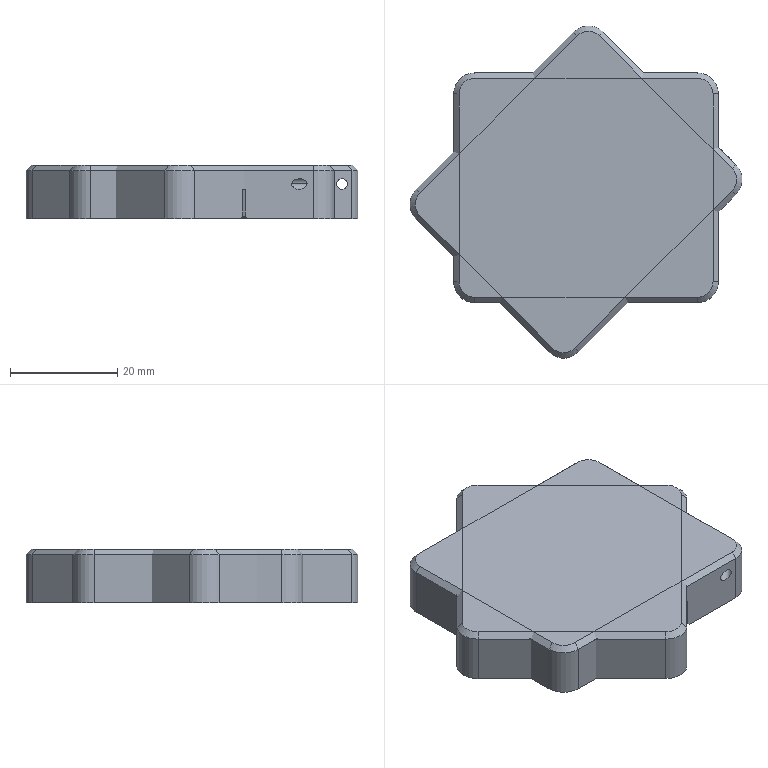NC program | NX | posted with a generic post | part box 61.954 x 61.954 x 10 mm
Whole program:
N10 G17 G21 G94 G90
(DRILLING , TOOL : D2开粗)
N12 T06 M6
N14 G54
N16 G17 G0 G90 X-2.999 Y6.5 B0. C0. S3000 M3
N18 G43 Z5.849 H6
N20 G94 G81 G99 Z-0.151 F30. R5.849
N22 G80
N24 M5
(DRILLING_COPY , TOOL : D2钻头)
N26 T07 M6
N28 G54
N30 G17 G0 G90 X-2.999 Y6.5 B0. C0. S3000 M3
N32 G43 Z5.849 H7
N34 G94 G83 G99 Z-10.151 F30. Q1.5 R5.849
N36 G80
N38 M5
N40 M2